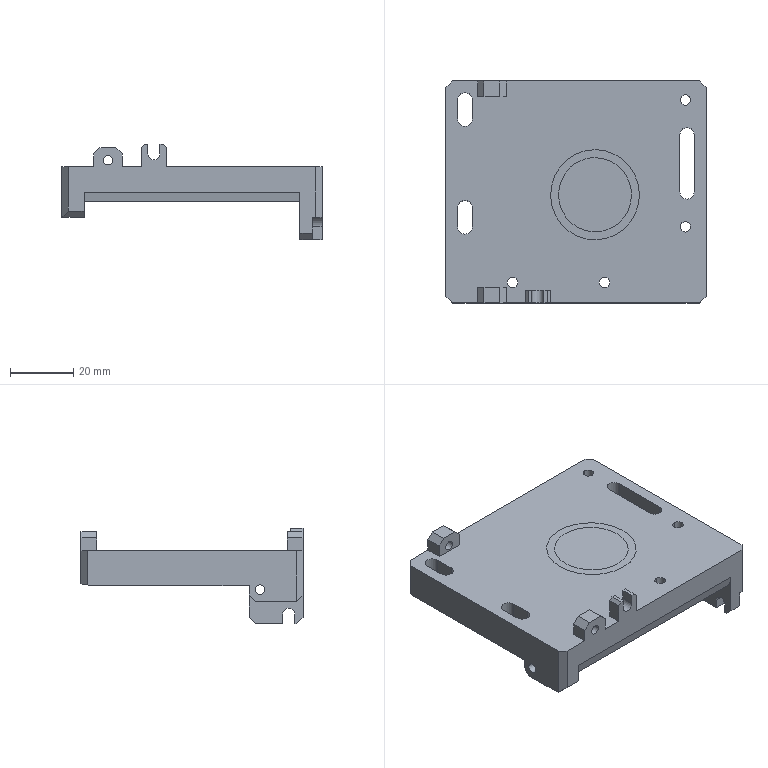NC program | NX | posted with a generic post | part box 82 x 70 x 30 mm
Lines 1 to 2138 of 2435, first 1715 of 2122 lines:
N10 G17 G21 G94 G90
(FLOOR_WALL , TOOL : D10JING)
N12 T11 M6
N14 G54
N16 G17 G0 G90 X45. Y-42.997 B0. C0. S9500 M3
N18 G43 Z30. H11
N20 Z3.
N22 G94 G1 Z0. F1250.
N24 X42.
N26 X-42.
N28 Y-38.174
N30 X42.
N32 Y-33.35
N34 X-42.
N36 Y-28.527
N38 X42.
N40 Y-23.704
N42 X-42.
N44 Y-18.88
N46 X42.
N48 Y-14.057
N50 X-42.
N52 Y-9.234
N54 X42.
N56 Y-4.41
N58 X-42.
N60 Y0.413
N62 X42.
N64 Y5.237
N66 X-42.
N68 Y10.06
N70 X42.
N72 Y14.883
N74 X-42.
N76 Y19.707
N78 X42.
N80 Y24.53
N82 X-42.
N84 Y29.353
N86 X42.
N88 Y34.177
N90 X-42.
N92 Y39.
N94 X42.
N96 X45.
N98 Z3.
N100 G0 Z30.
N102 M5
(FLOOR_WALL_1 , TOOL : D10JING)
N104 M6
N106 G54
N108 G17 G0 G90 X39.14 Y28.025 B0. C0. S9500 M3
N110 G43 Z30. H11
N112 Z-5.5
N114 G94 G1 Z-7. F1250.
N116 X38.866 Y28.5
N118 G3 X38. Y29. R1.
N120 G1 X15.
N122 Y33.
N124 X38.
N126 Y37.
N128 X15.
N130 G3 X14.134 Y36.5 R1.
N132 G1 X13.5 Y35.402
N134 Z-5.5
N136 G0 Z30.
N138 X-38.14 Y46.975
N140 Z-10.5
N142 G1 Z-12.
N144 X-37.866 Y46.5
N146 G3 X-37. Y46. R1.
N148 G1 X12.5
N150 Y41.118
N152 X-37.
N154 Y36.235
N156 X12.5
N158 Y31.353
N160 X-37.
N162 Y26.471
N164 X39.471
N166 Y21.588
N168 X-37.
N170 Y16.706
N172 X39.471
N174 Y11.824
N176 X-37.
N178 Y6.941
N180 X39.471
N182 Y2.059
N184 X-37.
N186 Y-2.824
N188 X39.471
N190 Y-7.706
N192 X-37.
N194 Y-12.588
N196 X39.471
N198 Y-17.471
N200 X-37.
N202 Y-22.353
N204 X39.471
N206 Y-27.235
N208 X-37.
N210 Y-32.118
N212 X12.5
N214 Y-37.
N216 X-37.
N218 Y-41.882
N220 X12.5
N222 G3 X12. Y-41.016 R1.
N224 G1 Z-10.5
N226 G0 Z-1.9
N228 X11.402 Y-47.5
N230 Z-10.5
N232 G1 Z-12.
N234 X12.5 Y-46.866
N236 G3 X13. Y-46. R1.
N238 G1 Y-29.
N240 X39.471
N242 G3 X40.337 Y-28.5 R1.
N244 G1 X40.971 Y-27.402
N246 Z-10.5
N248 G0 Z-1.9
N250 Y27.402
N252 Z-10.5
N254 G1 Z-12.
N256 X40.337 Y28.5
N258 G3 X39.471 Y29. R1.
N260 G1 X13.
N262 Y46.
N264 G3 X12.5 Y46.866 R1.
N266 G1 X11.402 Y47.5
N268 Z-10.5
N270 G0 Z30.
N272 X32.14 Y-46.975
N274 Z1.5
N276 G1 Z0.
N278 X31.866 Y-46.5
N280 G3 X31. Y-46. R1.
N282 G1 X15.
N284 Y-42.
N286 X38.
N288 Y-38.
N290 X15.
N292 G3 X14.134 Y-38.5 R1.
N294 G1 X13.5 Y-39.598
N296 Z1.5
N298 G0 Z30.
N300 X34.671 Y-43.5
N302 Z-5.4
N304 G1 X37.571 Z-6.177
N306 X34.5 Z-7.
N308 X37.571
N310 G2 X38.437 Y-44. R1.
N312 G1 X38.726 Y-44.5
N314 Z-5.5
N316 G0 Z3.1
N318 X39.514
N320 Z-5.5
N322 G1 Z-7.
N324 X38.937 Y-43.5
N326 G3 X38.071 Y-43. R1.
N328 G1 X34.
N330 Y-46.
N332 G3 X34.5 Y-46.866 R1.
N334 G1 X35.5 Y-47.443
N336 Z-5.5
N338 G0 Z30.
(ZLEVEL_PROFILE_COPY , TOOL : D10JING)
N340 X41.809 Y40.622
N342 Z-13.5
N344 G1 Z-15. F1000.
N346 X40.5 Y39.866
N348 G3 X40. Y39. R1.
N350 G1 Y-39. F1200.
N352 G2 X38.536 Y-42.536 R5.
N354 G1 X36.536 Y-44.536
N356 G2 X33. Y-46. R5.
N358 G1 X-33.
N360 G2 X-36.536 Y-44.536 R5.
N362 G1 X-38.536 Y-42.536
N364 G2 X-40. Y-39. R5.
N366 G1 Y39.
N368 G2 X-38.536 Y42.536 R5.
N370 G1 X-36.536 Y44.536
N372 G2 X-33. Y46. R5.
N374 G1 X33.
N376 G2 X36.536 Y44.536 R5.
N378 G1 X38.536 Y42.536
N380 G2 X40. Y39. R5.
N382 G3 X40.5 Y38.134 R1.
N384 G1 X42. Y37.268
N386 Z-13.5
N388 G0 Z30.
N390 X41.809 Y40.622
N392 Z-28.5
N394 G1 Z-30. F1000.
N396 X40.5 Y39.866
N398 G3 X40. Y39. R1.
N400 G1 Y-39. F1200.
N402 G2 X38.536 Y-42.536 R5.
N404 G1 X36.536 Y-44.536
N406 G2 X33. Y-46. R5.
N408 G1 X-33.
N410 G2 X-36.536 Y-44.536 R5.
N412 G1 X-38.536 Y-42.536
N414 G2 X-40. Y-39. R5.
N416 G1 Y39.
N418 G2 X-38.536 Y42.536 R5.
N420 G1 X-36.536 Y44.536
N422 G2 X-33. Y46. R5.
N424 G1 X33.
N426 G2 X36.536 Y44.536 R5.
N428 G1 X38.536 Y42.536
N430 G2 X40. Y39. R5.
N432 G3 X40.5 Y38.134 R1.
N434 G1 X42. Y37.268
N436 Z-28.5
N438 G0 Z30.
N440 M5
(ZLEVEL_PROFILE_COPY_1_COPY , TOOL : D3)
N442 T03 M6
N444 G54
N446 G17 G0 G90 X21. Y-1.698 B0. C0. S9500 M3
N448 G43 Z30. H3
N450 Z-10.5
N452 G94 G1 Y-32.5 Z-12.114 F1000.
N454 X22. Z-12.167
N456 Y32.5 F1200.
N458 X21.
N460 Y-32.5
N462 X22.
N464 Y-22.952 Z-12.333
N466 Y32.5
N468 X21.
N470 Y-32.5
N472 X22.
N474 Y-22.952 Z-12.5
N476 Y32.5
N478 X21.
N480 Y-32.5
N482 X22.
N484 Y-22.952
N486 G3 X21.85 Y-22.692 R0.3
N488 G1 X21.8 Y-22.663
N490 Z-12.2
N492 G0 Z30.
(CAVITY_MILL_COPY , TOOL : D3)
N494 X28.813 Y-41.189
N496 Z1.3
N498 G1 Z-0.2 F1000.
N500 X28.847 Y-40.788
N502 G2 X29.419 Y-39.968 R1.
N504 X31.56 Y-39.807 R3.02 F1100.
N506 G3 X32.178 Y-39.483 R0.5
N508 G2 X30.9 Y-38. R1.5
N510 G1 Y-34.
N512 G2 X32.114 Y-32.528 R1.5
N514 G3 X31.483 Y-32.231 R0.5
N516 G2 X29.517 Y-32.231 R3.02
N518 G3 X28.886 Y-32.528 R0.5
N520 G2 X30.1 Y-34. R1.5
N522 G1 Y-38.
N524 G2 X28.6 Y-39.5 R1.5
N526 G1 X27.499
N528 X27.5 Y-39.536
N530 Y-41.
N532 G2 X27.282 Y-41.778 R1.5
N534 G3 X27.926 Y-41.511 R0.5
N536 G2 X29.419 Y-39.968 R3.02
N538 X30.416 Y-40.053 R1.
N540 G1 X30.745 Y-40.283
N542 Z1.3
N544 G0 X28.813 Y-41.189 Z1.1
N546 G1 Z-0.4 F1000.
N548 X28.847 Y-40.788
N550 G2 X29.419 Y-39.968 R1.
N552 X31.56 Y-39.807 R3.02 F1100.
N554 G3 X32.178 Y-39.483 R0.5
N556 G2 X30.9 Y-38. R1.5
N558 G1 Y-34.
N560 G2 X32.114 Y-32.528 R1.5
N562 G3 X31.483 Y-32.231 R0.5
N564 G2 X29.517 Y-32.231 R3.02
N566 G3 X28.886 Y-32.528 R0.5
N568 G2 X30.1 Y-34. R1.5
N570 G1 Y-38.
N572 G2 X28.6 Y-39.5 R1.5
N574 G1 X27.5
N576 Y-39.536
N578 Y-41.
N580 G2 X27.282 Y-41.778 R1.5
N582 G3 X27.926 Y-41.511 R0.5
N584 G2 X29.419 Y-39.968 R3.02
N586 X30.416 Y-40.053 R1.
N588 G1 X30.745 Y-40.283
N590 Z1.1
N592 G0 X28.813 Y-41.189 Z0.9
N594 G1 Z-0.6 F1000.
N596 X28.847 Y-40.788
N598 G2 X29.419 Y-39.968 R1.
N600 X31.56 Y-39.807 R3.02 F1100.
N602 G3 X32.178 Y-39.483 R0.5
N604 G2 X30.9 Y-38. R1.5
N606 G1 Y-34.
N608 G2 X32.114 Y-32.528 R1.5
N610 G3 X31.483 Y-32.231 R0.5
N612 G2 X29.517 Y-32.231 R3.02
N614 G3 X28.886 Y-32.528 R0.5
N616 G2 X30.1 Y-34. R1.5
N618 G1 Y-38.
N620 G2 X28.6 Y-39.5 R1.5
N622 G1 X27.5
N624 Y-41.
N626 G2 X27.282 Y-41.778 R1.5
N628 G3 X27.926 Y-41.511 R0.5
N630 G2 X29.419 Y-39.968 R3.02
N632 X30.416 Y-40.053 R1.
N634 G1 X30.745 Y-40.283
N636 Z0.9
N638 G0 X28.813 Y-41.189 Z0.7
N640 G1 Z-0.8 F1000.
N642 X28.847 Y-40.788
N644 G2 X29.419 Y-39.968 R1.
N646 X31.56 Y-39.807 R3.02 F1100.
N648 G3 X32.178 Y-39.483 R0.5
N650 G2 X30.9 Y-38. R1.5
N652 G1 Y-34.
N654 G2 X32.114 Y-32.528 R1.5
N656 G3 X31.483 Y-32.231 R0.5
N658 G2 X29.517 Y-32.231 R3.02
N660 G3 X28.886 Y-32.528 R0.5
N662 G2 X30.1 Y-34. R1.5
N664 G1 Y-38.
N666 G2 X28.6 Y-39.5 R1.5
N668 G1 X27.5
N670 Y-41.
N672 G2 X27.282 Y-41.778 R1.5
N674 G3 X27.926 Y-41.511 R0.5
N676 G2 X29.419 Y-39.968 R3.02
N678 X30.416 Y-40.053 R1.
N680 G1 X30.745 Y-40.283
N682 Z0.7
N684 G0 X28.813 Y-41.189 Z0.5
N686 G1 Z-1. F1000.
N688 X28.847 Y-40.788
N690 G2 X29.419 Y-39.968 R1.
N692 X31.56 Y-39.807 R3.02 F1100.
N694 G3 X32.178 Y-39.483 R0.5
N696 G2 X30.9 Y-38. R1.5
N698 G1 Y-34.
N700 G2 X32.114 Y-32.528 R1.5
N702 G3 X31.483 Y-32.231 R0.5
N704 G2 X29.517 Y-32.231 R3.02
N706 G3 X28.886 Y-32.528 R0.5
N708 G2 X30.1 Y-34. R1.5
N710 G1 Y-38.
N712 G2 X28.6 Y-39.5 R1.5
N714 G1 X27.5
N716 Y-41.
N718 G2 X27.282 Y-41.778 R1.5
N720 G3 X27.926 Y-41.511 R0.5
N722 G2 X29.419 Y-39.968 R3.02
N724 X30.416 Y-40.053 R1.
N726 G1 X30.745 Y-40.283
N728 Z0.5
N730 G0 X28.813 Y-41.189 Z0.3
N732 G1 Z-1.2 F1000.
N734 X28.847 Y-40.788
N736 G2 X29.419 Y-39.968 R1.
N738 X31.56 Y-39.807 R3.02 F1100.
N740 G3 X32.178 Y-39.483 R0.5
N742 G2 X30.9 Y-38. R1.5
N744 G1 Y-34.
N746 G2 X32.114 Y-32.528 R1.5
N748 G3 X31.483 Y-32.231 R0.5
N750 G2 X29.517 Y-32.231 R3.02
N752 G3 X28.886 Y-32.528 R0.5
N754 G2 X30.1 Y-34. R1.5
N756 G1 Y-38.
N758 G2 X28.6 Y-39.5 R1.5
N760 G1 X27.5
N762 Y-41.
N764 G2 X27.282 Y-41.778 R1.5
N766 G3 X27.926 Y-41.511 R0.5
N768 G2 X29.419 Y-39.968 R3.02
N770 X30.416 Y-40.053 R1.
N772 G1 X30.745 Y-40.283
N774 Z0.3
N776 G0 X28.813 Y-41.189 Z0.1
N778 G1 Z-1.4 F1000.
N780 X28.847 Y-40.788
N782 G2 X29.419 Y-39.968 R1.
N784 X31.56 Y-39.807 R3.02 F1100.
N786 G3 X32.178 Y-39.483 R0.5
N788 G2 X30.9 Y-38. R1.5
N790 G1 Y-34.
N792 G2 X32.114 Y-32.528 R1.5
N794 G3 X31.483 Y-32.231 R0.5
N796 G2 X29.517 Y-32.231 R3.02
N798 G3 X28.886 Y-32.528 R0.5
N800 G2 X30.1 Y-34. R1.5
N802 G1 Y-38.
N804 G2 X28.6 Y-39.5 R1.5
N806 G1 X27.5
N808 Y-41.
N810 G2 X27.282 Y-41.778 R1.5
N812 G3 X27.926 Y-41.511 R0.5
N814 G2 X29.419 Y-39.968 R3.02
N816 X30.416 Y-40.053 R1.
N818 G1 X30.745 Y-40.283
N820 Z0.1
N822 G0 X28.813 Y-41.189 Z-0.1
N824 G1 Z-1.6 F1000.
N826 X28.847 Y-40.788
N828 G2 X29.419 Y-39.968 R1.
N830 X31.56 Y-39.807 R3.02 F1100.
N832 G3 X32.178 Y-39.483 R0.5
N834 G2 X30.9 Y-38. R1.5
N836 G1 Y-34.
N838 G2 X32.114 Y-32.528 R1.5
N840 G3 X31.483 Y-32.231 R0.5
N842 G2 X29.517 Y-32.231 R3.02
N844 G3 X28.886 Y-32.528 R0.5
N846 G2 X30.1 Y-34. R1.5
N848 G1 Y-38.
N850 G2 X28.6 Y-39.5 R1.5
N852 G1 X27.503
N854 X27.5 Y-39.536
N856 Y-41.
N858 G2 X27.282 Y-41.778 R1.5
N860 G3 X27.926 Y-41.511 R0.5
N862 G2 X29.419 Y-39.968 R3.02
N864 X30.416 Y-40.053 R1.
N866 G1 X30.745 Y-40.283
N868 Z-0.1
N870 G0 X28.813 Y-41.189 Z-0.3
N872 G1 Z-1.8 F1000.
N874 X28.847 Y-40.788
N876 G2 X29.419 Y-39.968 R1.
N878 X31.56 Y-39.807 R3.02 F1100.
N880 G3 X32.178 Y-39.483 R0.5
N882 G2 X30.9 Y-38. R1.5
N884 G1 Y-34.
N886 G2 X32.114 Y-32.528 R1.5
N888 G3 X31.483 Y-32.231 R0.5
N890 G2 X29.517 Y-32.231 R3.02
N892 G3 X28.886 Y-32.528 R0.5
N894 G2 X30.1 Y-34. R1.5
N896 G1 Y-38.
N898 G2 X28.6 Y-39.5 R1.5
N900 G1 X27.504
N902 X27.5 Y-39.536
N904 Y-41.
N906 G2 X27.282 Y-41.778 R1.5
N908 G3 X27.926 Y-41.511 R0.5
N910 G2 X29.419 Y-39.968 R3.02
N912 X30.416 Y-40.053 R1.
N914 G1 X30.745 Y-40.283
N916 Z-0.3
N918 G0 X28.813 Y-41.189 Z-0.5
N920 G1 Z-2. F1000.
N922 X28.847 Y-40.788
N924 G2 X29.419 Y-39.968 R1.
N926 X31.56 Y-39.807 R3.02 F1100.
N928 G3 X32.178 Y-39.483 R0.5
N930 G2 X30.9 Y-38. R1.5
N932 G1 Y-34.
N934 G2 X32.114 Y-32.528 R1.5
N936 G3 X31.483 Y-32.231 R0.5
N938 G2 X29.517 Y-32.231 R3.02
N940 G3 X28.886 Y-32.528 R0.5
N942 G2 X30.1 Y-34. R1.5
N944 G1 Y-38.
N946 G2 X28.6 Y-39.5 R1.5
N948 G1 X27.505
N950 X27.5 Y-39.536
N952 Y-41.
N954 G2 X27.282 Y-41.778 R1.5
N956 G3 X27.926 Y-41.511 R0.5
N958 G2 X29.419 Y-39.968 R3.02
N960 X30.416 Y-40.053 R1.
N962 G1 X30.745 Y-40.283
N964 Z-0.5
N966 G0 X28.813 Y-41.189 Z-0.7
N968 G1 Z-2.2 F1000.
N970 X28.847 Y-40.788
N972 G2 X29.419 Y-39.968 R1.
N974 X31.56 Y-39.807 R3.02 F1100.
N976 G3 X32.178 Y-39.483 R0.5
N978 G2 X30.9 Y-38. R1.5
N980 G1 Y-34.
N982 G2 X32.114 Y-32.528 R1.5
N984 G3 X31.483 Y-32.231 R0.5
N986 G2 X29.517 Y-32.231 R3.02
N988 G3 X28.886 Y-32.528 R0.5
N990 G2 X30.1 Y-34. R1.5
N992 G1 Y-38.
N994 G2 X28.6 Y-39.5 R1.5
N996 G1 X27.506
N998 X27.5 Y-39.536
N1000 Y-41.
N1002 G2 X27.282 Y-41.778 R1.5
N1004 G3 X27.926 Y-41.511 R0.5
N1006 G2 X29.419 Y-39.968 R3.02
N1008 X30.416 Y-40.053 R1.
N1010 G1 X30.745 Y-40.283
N1012 Z-0.7
N1014 G0 X28.813 Y-41.189 Z-0.9
N1016 G1 Z-2.4 F1000.
N1018 X28.847 Y-40.788
N1020 G2 X29.419 Y-39.968 R1.
N1022 X31.56 Y-39.807 R3.02 F1100.
N1024 G3 X32.178 Y-39.483 R0.5
N1026 G2 X30.9 Y-38. R1.5
N1028 G1 Y-34.
N1030 G2 X32.114 Y-32.528 R1.5
N1032 G3 X31.483 Y-32.231 R0.5
N1034 G2 X29.517 Y-32.231 R3.02
N1036 G3 X28.886 Y-32.528 R0.5
N1038 G2 X30.1 Y-34. R1.5
N1040 G1 Y-38.
N1042 G2 X28.6 Y-39.5 R1.5
N1044 G1 X27.5
N1046 Y-41.
N1048 G2 X27.282 Y-41.778 R1.5
N1050 G3 X27.926 Y-41.511 R0.5
N1052 G2 X29.419 Y-39.968 R3.02
N1054 X30.416 Y-40.053 R1.
N1056 G1 X30.745 Y-40.283
N1058 Z-0.9
N1060 G0 X28.813 Y-41.189 Z-1.1
N1062 G1 Z-2.6 F1000.
N1064 X28.847 Y-40.788
N1066 G2 X29.419 Y-39.968 R1.
N1068 X31.56 Y-39.807 R3.02 F1100.
N1070 G3 X32.178 Y-39.483 R0.5
N1072 G2 X30.9 Y-38. R1.5
N1074 G1 Y-34.
N1076 G2 X32.114 Y-32.528 R1.5
N1078 G3 X31.483 Y-32.231 R0.5
N1080 G2 X29.517 Y-32.231 R3.02
N1082 G3 X28.886 Y-32.528 R0.5
N1084 G2 X30.1 Y-34. R1.5
N1086 G1 Y-38.
N1088 G2 X28.6 Y-39.5 R1.5
N1090 G1 X27.5
N1092 Y-41.
N1094 G2 X27.282 Y-41.778 R1.5
N1096 G3 X27.926 Y-41.511 R0.5
N1098 G2 X29.419 Y-39.968 R3.02
N1100 X30.416 Y-40.053 R1.
N1102 G1 X30.745 Y-40.283
N1104 Z-1.1
N1106 G0 X28.813 Y-41.189 Z-1.3
N1108 G1 Z-2.8 F1000.
N1110 X28.847 Y-40.788
N1112 G2 X29.419 Y-39.968 R1.
N1114 X31.56 Y-39.807 R3.02 F1100.
N1116 G3 X32.178 Y-39.483 R0.5
N1118 G2 X30.9 Y-38. R1.5
N1120 G1 Y-34.
N1122 G2 X32.114 Y-32.528 R1.5
N1124 G3 X31.483 Y-32.231 R0.5
N1126 G2 X29.517 Y-32.231 R3.02
N1128 G3 X28.886 Y-32.528 R0.5
N1130 G2 X30.1 Y-34. R1.5
N1132 G1 Y-38.
N1134 G2 X28.6 Y-39.5 R1.5
N1136 G1 X27.5
N1138 Y-41.
N1140 G2 X27.282 Y-41.778 R1.5
N1142 G3 X27.926 Y-41.511 R0.5
N1144 G2 X29.419 Y-39.968 R3.02
N1146 X30.416 Y-40.053 R1.
N1148 G1 X30.745 Y-40.283
N1150 Z-1.3
N1152 G0 X28.813 Y-41.189 Z-1.5
N1154 G1 Z-3. F1000.
N1156 X28.847 Y-40.788
N1158 G2 X29.419 Y-39.968 R1.
N1160 X31.56 Y-39.807 R3.02 F1100.
N1162 G3 X32.178 Y-39.483 R0.5
N1164 G2 X30.9 Y-38. R1.5
N1166 G1 Y-34.
N1168 G2 X32.114 Y-32.528 R1.5
N1170 G3 X31.483 Y-32.231 R0.5
N1172 G2 X29.517 Y-32.231 R3.02
N1174 G3 X28.886 Y-32.528 R0.5
N1176 G2 X30.1 Y-34. R1.5
N1178 G1 Y-38.
N1180 G2 X28.6 Y-39.5 R1.5
N1182 G1 X27.5
N1184 Y-41.
N1186 G2 X27.282 Y-41.778 R1.5
N1188 G3 X27.926 Y-41.511 R0.5
N1190 G2 X29.419 Y-39.968 R3.02
N1192 X30.416 Y-40.053 R1.
N1194 G1 X30.745 Y-40.283
N1196 Z-1.5
N1198 G0 X28.813 Y-41.193 Z-1.7
N1200 G1 Z-3.2 F1000.
N1202 X28.848 Y-40.793
N1204 G2 X29.422 Y-39.974 R1.
N1206 X31.458 Y-39.788 R3.02 F1100.
N1208 G1 X31.556 Y-39.815
N1210 G3 X32.171 Y-39.486 R0.5
N1212 G2 X30.889 Y-38. R1.487
N1214 G1 Y-34.
N1216 G2 X32.088 Y-32.528 R1.486
N1218 G3 X31.462 Y-32.232 R0.5
N1220 G2 X29.945 Y-32.337 R3.02
N1222 X29.534 Y-32.231 R3.02
N1224 G3 X28.907 Y-32.53 R0.5
N1226 G2 X30.099 Y-33.827 R1.475
N1228 G1 X30.117 Y-33.999
N1230 X30.111 Y-34.02
N1232 Y-38.
N1234 G2 X28.6 Y-39.5 R1.483
N1236 G1 X27.5
N1238 Y-41.
N1240 G2 X27.281 Y-41.781 R1.5
N1242 G3 X27.925 Y-41.514 R0.5
N1244 G2 X29.422 Y-39.974 R3.02
N1246 X30.418 Y-40.061 R1.
N1248 G1 X30.747 Y-40.292
N1250 Z-1.7
N1252 G0 X28.813 Y-41.196 Z-1.9
N1254 G1 Z-3.4 F1000.
N1256 X28.849 Y-40.796
N1258 G2 X29.424 Y-39.978 R1.
N1260 X31.52 Y-39.812 R3.02 F1100.
N1262 G3 X32.132 Y-39.485 R0.5
N1264 G2 X30.894 Y-38.349 R1.496
N1266 G1 X30.85 Y-38.105
N1268 X30.857 Y-38.
N1270 Y-34.011
N1272 X30.846 Y-33.988
N1274 G2 X31.374 Y-32.863 R1.55
N1276 G1 X31.553 Y-32.731
N1278 G2 X32.093 Y-32.516 R1.324
N1280 G3 X31.464 Y-32.212 R0.5
N1282 G2 X29.533 Y-32.21 R3.02
N1284 G3 X28.9 Y-32.519 R0.5
N1286 G2 X30.143 Y-34.033 R1.49
N1288 G1 Y-38.
N1290 G2 X28.713 Y-39.499 R1.482
N1292 G1 X28.6 Y-39.5
N1294 X27.5
N1296 Y-41.
N1298 G2 X27.28 Y-41.782 R1.5
N1300 G3 X27.925 Y-41.517 R0.5
N1302 G2 X29.424 Y-39.978 R3.02
N1304 X30.42 Y-40.067 R1.
N1306 G1 X30.749 Y-40.298
N1308 Z-1.9
N1310 G0 X28.814 Y-41.206 Z-2.1
N1312 G1 Z-3.6 F1000.
N1314 X28.851 Y-40.806
N1316 G2 X29.43 Y-39.99 R1.
N1318 X31.483 Y-39.821 R3.02 F1100.
N1320 G3 X32.091 Y-39.487 R0.5
N1322 G2 X30.835 Y-38.349 R1.495
N1324 G1 X30.798 Y-38.105
N1326 X30.803 Y-38.
N1328 Y-34.029
N1330 X30.794 Y-33.993
N1332 G2 X30.886 Y-33.489 R1.196
N1334 X32.044 Y-32.52 R1.489
N1336 G3 X31.42 Y-32.207 R0.5
N1338 G2 X29.582 Y-32.207 R3.02
N1340 G3 X28.957 Y-32.52 R0.5
N1342 G2 X30.153 Y-33.621 R1.483
N1344 G1 X30.184 Y-33.708
N1346 G2 X30.206 Y-34. R2.036
N1348 G1 X30.197 Y-34.03
N1350 Y-38.
N1352 X30.202 Y-38.105
N1354 G2 X30.153 Y-38.39 R0.68
N1356 X28.706 Y-39.5 R1.489
N1358 G1 X27.5
N1360 Y-41.
N1362 G2 X27.277 Y-41.787 R1.5
N1364 G3 X27.923 Y-41.524 R0.5
N1366 G2 X29.43 Y-39.99 R3.02
N1368 X30.425 Y-40.083 R1.
N1370 G1 X30.753 Y-40.316
N1372 Z-2.1
N1374 G0 X28.814 Y-41.218 Z-2.3
N1376 G1 Z-3.8 F1000.
N1378 X28.854 Y-40.819
N1380 G2 X29.437 Y-40.006 R1.
N1382 X31.437 Y-39.835 R3.02 F1100.
N1384 G3 X32.042 Y-39.49 R0.5
N1386 G2 X30.717 Y-37.965 R1.498
N1388 G1 X30.723 Y-37.948
N1390 Y-34.049
N1392 X30.717 Y-34.037
N1394 X30.714 Y-33.952
N1396 G2 X31.988 Y-32.517 R1.501
N1398 G3 X31.37 Y-32.195 R0.5
N1400 G2 X29.629 Y-32.194 R3.02
N1402 G3 X29.01 Y-32.517 R0.5
N1404 G2 X30.184 Y-33.464 R1.493
N1406 G1 X30.261 Y-33.708
N1408 G2 X30.284 Y-33.996 R1.975
N1410 G1 X30.277 Y-34.037
N1412 Y-37.949
N1414 X30.283 Y-37.966
N1416 G2 X30.161 Y-38.593 R1.286
N1418 X28.784 Y-39.5 R1.496
N1420 G1 X27.5
N1422 Y-41.
N1424 G2 X27.273 Y-41.793 R1.5
N1426 G3 X27.92 Y-41.534 R0.5
N1428 G2 X29.437 Y-40.006 R3.02
N1430 X30.432 Y-40.106 R1.
N1432 G1 X30.758 Y-40.34
N1434 Z-2.3
N1436 G0 X28.814 Y-41.235 Z-2.5
N1438 G1 Z-4. F1000.
N1440 X28.857 Y-40.836
N1442 G2 X29.447 Y-40.028 R1.
N1444 X31.369 Y-39.853 R3.02 F1100.
N1446 G3 X31.968 Y-39.494 R0.5
N1448 G2 X30.61 Y-37.965 R1.493
N1450 G1 X30.616 Y-37.948
N1452 Y-34.049
N1454 X30.61 Y-34.037
N1456 G2 X30.702 Y-33.464 R1.679
N1458 X31.921 Y-32.512 R1.51
N1460 G3 X31.309 Y-32.174 R0.5
N1462 G2 X29.697 Y-32.175 R3.02
N1464 G3 X29.085 Y-32.512 R0.5
N1466 G2 X30.39 Y-34.021 R1.493
N1468 G1 X30.384 Y-34.032
N1470 Y-37.948
N1472 X30.39 Y-37.965
N1474 G2 X28.89 Y-39.5 R1.496
N1476 G1 X27.507
N1478 X27.5 Y-39.522
N1480 Y-41.
N1482 G2 X27.268 Y-41.802 R1.5
N1484 G3 X27.916 Y-41.547 R0.5
N1486 G2 X29.447 Y-40.028 R3.02
N1488 X30.441 Y-40.135 R1.
N1490 G1 X30.765 Y-40.372
N1492 Z-2.5
N1494 G0 X32.749 Y-40.1 Z-2.7
N1496 G1 Z-4.2 F1000.
N1498 X32.721 Y-40.044
N1500 G3 X31.883 Y-39.498 R1.
N1502 G2 X30.5 Y-38.337 R1.505 F1100.
N1504 X29.039 Y-39.5 R1.504
N1506 G1 X27.507
N1508 Y-40.973
N1510 X27.513 Y-40.985
N1512 X27.486 Y-41.28
N1514 X27.468 Y-41.352
N1516 G2 X27.27 Y-41.82 R1.456
N1518 G3 X27.185 Y-42.742 R1.
N1520 G1 Z-2.7
N1522 G0 X32.639 Y-40.1 Z-2.9
N1524 G1 Z-4.4 F1000.
N1526 X32.596 Y-40.021
N1528 G3 X31.743 Y-39.5 R1.
N1530 G2 X30.502 Y-38.792 R1.509 F1100.
N1532 X29.225 Y-39.5 R1.518
N1534 G1 X27.527
N1536 Y-40.984
N1538 G2 X27.292 Y-41.818 R1.478
N1540 G3 X27.209 Y-42.742 R1.
N1542 G1 Z-2.9
N1544 G0 X32.481 Y-40.1 Z-3.1
N1546 G1 Z-4.6 F1000.
N1548 X32.423 Y-40.
N1550 G3 X31.557 Y-39.5 R1.
N1552 G1 X31.518 F1100.
N1554 G2 X30.502 Y-39.101 R1.476
N1556 X29.482 Y-39.5 R1.511
N1558 G1 X27.561
N1560 Y-40.969
N1562 X27.568 Y-41.036
N1564 G2 X27.314 Y-41.838 R1.498
N1566 G3 X27.213 Y-42.762 R1.
N1568 G1 Z-3.1
N1570 G0 X32.192 Y-40.1 Z-3.3
N1572 G1 Z-4.8 F1000.
N1574 X32.134 Y-40.
N1576 G3 X31.268 Y-39.5 R1.
N1578 G1 X31.08 F1100.
N1580 G2 X30.502 Y-39.375 R1.423
N1582 X29.92 Y-39.5 R1.536
N1584 G1 X27.609
N1586 Y-40.978
N1588 X27.617 Y-41.036
N1590 X27.602 Y-41.175
N1592 G2 X27.34 Y-41.867 R1.489
N1594 G3 X27.22 Y-42.788 R1.
N1596 G1 Z-3.3
N1598 G0 X31.809 Y-40.1 Z-3.5
N1600 G1 Z-5. F1000.
N1602 X31.751 Y-40.
N1604 G3 X30.885 Y-39.5 R1.
N1606 G1 X27.672 F1100.
N1608 Y-40.961
N1610 X27.677 Y-40.988
N1612 G2 X27.413 Y-41.854 R1.494
N1614 G3 X27.302 Y-42.776 R1.
N1616 G1 Z-3.5
N1618 G0 X31.891 Y-40.1 Z-3.7
N1620 G1 Z-5.2 F1000.
N1622 X31.834 Y-40.
N1624 G3 X30.968 Y-39.5 R1.
N1626 G1 X27.75 F1100.
N1628 Y-41.
N1630 X27.76 Y-41.036
N1632 G2 X27.492 Y-41.856 R1.502
N1634 G3 X27.376 Y-42.779 R1.
N1636 G1 Z-3.7
N1638 G0 X31.981 Y-40.1 Z-3.9
N1640 G1 Z-5.4 F1000.
N1642 X31.923 Y-40.
N1644 G3 X31.057 Y-39.5 R1.
N1646 G1 X27.847 F1100.
N1648 Y-41.
N1650 G2 X27.589 Y-41.854 R1.482
N1652 G3 X27.481 Y-42.776 R1.
N1654 G1 Z-3.9
N1656 G0 X32.104 Y-40.1 Z-4.1
N1658 G1 Z-5.6 F1000.
N1660 X32.047 Y-40.
N1662 G3 X31.181 Y-39.5 R1.
N1664 G1 X27.962 F1100.
N1666 Y-41.
N1668 X27.973 Y-41.036
N1670 G2 X27.7 Y-41.86 R1.503
N1672 G3 X27.581 Y-42.783 R1.
N1674 G1 Z-4.1
N1676 G0 X32.247 Y-40.1 Z-4.3
N1678 G1 Z-5.8 F1000.
N1680 X32.189 Y-40.
N1682 G3 X31.323 Y-39.5 R1.
N1684 G1 X28.1 F1100.
N1686 Y-41.
N1688 G2 X27.797 Y-41.912 R1.487
N1690 G3 X27.643 Y-42.828 R1.
N1692 G1 Z-4.3
N1694 G0 X32.407 Y-40.1 Z-4.5
N1696 G1 Z-6. F1000.
N1698 X32.349 Y-40.
N1700 G3 X31.483 Y-39.5 R1.
N1702 G1 X28.264 F1100.
N1704 Y-40.974
N1706 X28.281 Y-41.036
N1708 G2 X28.2 Y-41.454 R1.102
N1710 X27.999 Y-41.863 R1.493
N1712 G3 X27.881 Y-42.785 R1.
N1714 G1 Z-4.5
N1716 G0 X32.604 Y-40.1 Z-4.7
N1718 G1 Z-6.2 F1000.
N1720 X32.546 Y-40.
N1722 G3 X31.68 Y-39.5 R1.
N1724 G1 X28.46 F1100.
N1726 Y-40.974
N1728 X28.47 Y-41.036
N1730 G2 X28.202 Y-41.859 R1.488
N1732 G3 X28.085 Y-42.78 R1.
N1734 G1 Z-4.7
N1736 G0 X32.837 Y-40.1 Z-4.9
N1738 G1 Z-6.4 F1000.
N1740 X32.78 Y-40.
N1742 G3 X31.914 Y-39.5 R1.
N1744 G1 X28.7 F1100.
N1746 Y-41.
N1748 G2 X28.438 Y-41.862 R1.478
N1750 G3 X28.326 Y-42.783 R1.
N1752 G1 Z-4.9
N1754 G0 X33.151 Y-40.1 Z-5.1
N1756 G1 Z-6.6 F1000.
N1758 X33.093 Y-40.
N1760 G3 X32.227 Y-39.5 R1.
N1762 G1 X29.003 F1100.
N1764 Y-40.974
N1766 X29.023 Y-41.036
N1768 G2 X28.808 Y-41.769 R1.535
N1770 G1 X28.754 Y-41.854
N1772 G3 X28.641 Y-42.776 R1.
N1774 G1 Z-5.1
N1776 G0 X33.583 Y-40.1 Z-5.3
N1778 G1 Z-6.8 F1000.
N1780 X33.525 Y-40.
N1782 G3 X32.659 Y-39.5 R1.
N1784 G1 X29.423 F1100.
N1786 Y-40.974
N1788 X29.449 Y-41.036
N1790 G2 X29.35 Y-41.524 R1.776
N1792 X29.146 Y-41.89 R1.534
N1794 G3 X28.996 Y-42.81 R1.
N1796 G1 Z-5.3
N1798 G0 X34.566 Y-40.1 Z-5.5
N1800 G1 Z-7. F1000.
N1802 X34.509 Y-40.
N1804 G3 X33.643 Y-39.5 R1.
N1806 G1 X30.378 F1100.
N1808 Y-41.
N1810 X30.406 Y-40.987
N1812 X30.435 Y-41.004
N1814 X30.436 Y-41.036
N1816 G2 X30.19 Y-41.814 R1.237
N1818 G3 X30.049 Y-42.753 R1.
N1820 G1 Z-5.5
N1822 G0 Z30.
N1824 X28.339 Y-31.9
N1826 Z-2.7
N1828 G1 Z-4.2 F1000.
N1830 X28.353 Y-31.931
N1832 G3 X29.172 Y-32.506 R1.
N1834 G2 X30.498 Y-33.666 R1.495 F1100.
N1836 X31.831 Y-32.506 R1.504
N1838 G3 X32.649 Y-31.931 R1.
N1840 G1 X32.664 Y-31.9
N1842 Z-2.7
N1844 G0 X28.456 Z-2.9
N1846 G1 Z-4.4 F1000.
N1848 X28.482 Y-31.952
N1850 G3 X29.317 Y-32.503 R1.
N1852 G2 X30.498 Y-33.209 R1.492 F1100.
N1854 X31.687 Y-32.503 R1.51
N1856 G3 X32.522 Y-31.952 R1.
N1858 G1 X32.548 Y-31.9
N1860 Z-2.9
N1862 G0 X28.572 Z-3.1
N1864 G1 Z-4.6 F1000.
N1866 X28.628 Y-31.997
N1868 G3 X29.492 Y-32.5 R1.
N1870 G2 X30.498 Y-32.897 R1.486 F1100.
N1872 X31.525 Y-32.5 R1.503
N1874 G3 X32.394 Y-32.005 R1.
N1876 G1 X32.456 Y-31.9
N1878 Z-3.1
N1880 G0 X28.82 Z-3.3
N1882 G1 Z-4.8 F1000.
N1884 X28.878 Y-32.
N1886 G3 X29.744 Y-32.5 R1.
N1888 G1 X29.92 F1100.
N1890 G2 X30.519 Y-32.609 R3.215
N1892 X31.08 Y-32.5 R1.862
N1894 G1 X31.235
N1896 G3 X32.101 Y-32. R1.
N1898 G1 X32.158 Y-31.9
N1900 Z-3.3
N1902 G0 Z30.
N1904 M5
(CAVITY_MILL_COPY_COPY_COPY , TOOL : D1.5)
N1906 T14 M6
N1908 G54
N1910 G17 G0 G90 X20.55 Y-31.46 B0. C0. S9500 M3
N1912 G43 Z30. H14
N1914 Z-10.6
N1916 G94 G1 Z-12.1 F1000.
N1918 G3 X20.25 Y-32.174 R1.
N1920 G1 Y-33. F1100.
N1922 G3 X20.5 Y-33.25 R0.25
N1924 G1 X21.326
N1926 G3 X21.576 Y-33.183 R0.5
N1928 G1 X21.5 Y-32.82
N1930 Z-10.6
N1932 G0 Z30.
N1934 X20.55 Y-31.46
N1936 Z-10.7
N1938 G1 Z-12.2 F1000.
N1940 G3 X20.25 Y-32.174 R1.
N1942 G1 Y-33. F1100.
N1944 G3 X20.5 Y-33.25 R0.25
N1946 G1 X21.326
N1948 G3 X21.576 Y-33.183 R0.5
N1950 G1 X21.5 Y-32.82
N1952 Z-10.7
N1954 G0 Z30.
N1956 X20.55 Y-31.46
N1958 Z-10.8
N1960 G1 Z-12.3 F1000.
N1962 G3 X20.25 Y-32.174 R1.
N1964 G1 Y-33. F1100.
N1966 G3 X20.5 Y-33.25 R0.25
N1968 G1 X21.326
N1970 G3 X21.576 Y-33.183 R0.5
N1972 G1 X21.5 Y-32.82
N1974 Z-10.8
N1976 G0 Z30.
N1978 X20.55 Y-31.46
N1980 Z-10.9
N1982 G1 Z-12.4 F1000.
N1984 G3 X20.25 Y-32.174 R1.
N1986 G1 Y-33. F1100.
N1988 G3 X20.5 Y-33.25 R0.25
N1990 G1 X21.326
N1992 G3 X21.576 Y-33.183 R0.5
N1994 G1 X21.5 Y-32.82
N1996 Z-10.9
N1998 G0 Z30.
N2000 X20.55 Y-31.46
N2002 Z-11.
N2004 G1 Z-12.5 F1000.
N2006 G3 X20.25 Y-32.174 R1.
N2008 G1 Y-33. F1100.
N2010 G3 X20.5 Y-33.25 R0.25
N2012 G1 X21.326
N2014 G3 X21.576 Y-33.183 R0.5
N2016 G1 X21.5 Y-32.82
N2018 Z-11.
N2020 G0 Z30.
N2022 X21.025 Y-32.475
N2024 Z-10.6
N2026 G1 Z-12.1 F1000.
N2028 X20.808 Y-32.75
N2030 G3 X21.674 Y-33.25 R1.
N2032 G1 X22.5 F1100.
N2034 G3 X22.75 Y-33. R0.25
N2036 G1 Y-32.174
N2038 G3 X22.45 Y-31.46 R1.
N2040 G1 Z-10.6
N2042 G0 Z30.
N2044 X21.025 Y-32.475
N2046 Z-10.7
N2048 G1 Z-12.2 F1000.
N2050 X20.808 Y-32.75
N2052 G3 X21.674 Y-33.25 R1.
N2054 G1 X22.5 F1100.
N2056 G3 X22.75 Y-33. R0.25
N2058 G1 Y-32.174
N2060 G3 X22.45 Y-31.46 R1.
N2062 G1 Z-10.7
N2064 G0 Z30.
N2066 X21.025 Y-32.475
N2068 Z-10.8
N2070 G1 Z-12.3 F1000.
N2072 X20.808 Y-32.75
N2074 G3 X21.674 Y-33.25 R1.
N2076 G1 X22.5 F1100.
N2078 G3 X22.75 Y-33. R0.25
N2080 G1 Y-32.174
N2082 G3 X22.45 Y-31.46 R1.
N2084 G1 Z-10.8
N2086 G0 Z30.
N2088 X21.025 Y-32.475
N2090 Z-10.9
N2092 G1 Z-12.4 F1000.
N2094 X20.808 Y-32.75
N2096 G3 X21.674 Y-33.25 R1.
N2098 G1 X22.5 F1100.
N2100 G3 X22.75 Y-33. R0.25
N2102 G1 Y-32.174
N2104 G3 X22.45 Y-31.46 R1.
N2106 G1 Z-10.9
N2108 G0 Z30.
N2110 X21.025 Y-32.475
N2112 Z-11.
N2114 G1 Z-12.5 F1000.
N2116 X20.808 Y-32.75
N2118 G3 X21.674 Y-33.25 R1.
N2120 G1 X22.5 F1100.
N2122 G3 X22.75 Y-33. R0.25
N2124 G1 Y-32.174
N2126 G3 X22.45 Y-31.46 R1.
N2128 G1 Z-11.
N2130 G0 Z30.
N2132 Y31.46
N2134 Z-10.6
N2136 G1 Z-12.1 F1000.
N2138 G3 X22.75 Y32.174 R1.
N2140 G1 Y33. F1100.
N2142 G3 X22.5 Y33.25 R0.25
N2144 G1 X21.674
N2146 G3 X21.424 Y33.183 R0.5
N2148 G1 X21.5 Y32.82
N2150 Z-10.6
N2152 G0 Z30.
N2154 X22.45 Y31.46
N2156 Z-10.7
N2158 G1 Z-12.2 F1000.
N2160 G3 X22.75 Y32.174 R1.
N2162 G1 Y33. F1100.
N2164 G3 X22.5 Y33.25 R0.25
N2166 G1 X21.674
N2168 G3 X21.424 Y33.183 R0.5
N2170 G1 X21.5 Y32.82
N2172 Z-10.7
N2174 G0 Z30.
N2176 X22.45 Y31.46
N2178 Z-10.8
N2180 G1 Z-12.3 F1000.
N2182 G3 X22.75 Y32.174 R1.
N2184 G1 Y33. F1100.
N2186 G3 X22.5 Y33.25 R0.25
N2188 G1 X21.674
N2190 G3 X21.424 Y33.183 R0.5
N2192 G1 X21.5 Y32.82
N2194 Z-10.8
N2196 G0 Z30.
N2198 X22.45 Y31.46
N2200 Z-10.9
N2202 G1 Z-12.4 F1000.
N2204 G3 X22.75 Y32.174 R1.
N2206 G1 Y33. F1100.
N2208 G3 X22.5 Y33.25 R0.25
N2210 G1 X21.674
N2212 G3 X21.424 Y33.183 R0.5
N2214 G1 X21.5 Y32.82
N2216 Z-10.9
N2218 G0 Z30.
N2220 X22.45 Y31.46
N2222 Z-11.
N2224 G1 Z-12.5 F1000.
N2226 G3 X22.75 Y32.174 R1.
N2228 G1 Y33. F1100.
N2230 G3 X22.5 Y33.25 R0.25
N2232 G1 X21.674
N2234 G3 X21.424 Y33.183 R0.5
N2236 G1 X21.5 Y32.82
N2238 Z-11.
N2240 G0 Z30.
N2242 X21.975 Y32.475
N2244 Z-10.6
N2246 G1 Z-12.1 F1000.
N2248 X22.192 Y32.75
N2250 G3 X21.326 Y33.25 R1.
N2252 G1 X20.5 F1100.
N2254 G3 X20.25 Y33. R0.25
N2256 G1 Y32.174
N2258 G3 X20.55 Y31.46 R1.
N2260 G1 Z-10.6
N2262 G0 Z30.
N2264 X21.975 Y32.475
N2266 Z-10.7
N2268 G1 Z-12.2 F1000.
N2270 X22.192 Y32.75
N2272 G3 X21.326 Y33.25 R1.
N2274 G1 X20.5 F1100.
N2276 G3 X20.25 Y33. R0.25
N2278 G1 Y32.174
N2280 G3 X20.55 Y31.46 R1.
N2282 G1 Z-10.7
N2284 G0 Z30.
N2286 X21.975 Y32.475
N2288 Z-10.8
N2290 G1 Z-12.3 F1000.
N2292 X22.192 Y32.75
N2294 G3 X21.326 Y33.25 R1.
N2296 G1 X20.5 F1100.
N2298 G3 X20.25 Y33. R0.25
N2300 G1 Y32.174
N2302 G3 X20.55 Y31.46 R1.
N2304 G1 Z-10.8
N2306 G0 Z30.
N2308 X21.975 Y32.475
N2310 Z-10.9
N2312 G1 Z-12.4 F1000.
N2314 X22.192 Y32.75
N2316 G3 X21.326 Y33.25 R1.
N2318 G1 X20.5 F1100.
N2320 G3 X20.25 Y33. R0.25
N2322 G1 Y32.174
N2324 G3 X20.55 Y31.46 R1.
N2326 G1 Z-10.9
N2328 G0 Z30.
N2330 X21.975 Y32.475
N2332 Z-11.
N2334 G1 Z-12.5 F1000.
N2336 X22.192 Y32.75
N2338 G3 X21.326 Y33.25 R1.
N2340 G1 X20.5 F1100.
N2342 G3 X20.25 Y33. R0.25
N2344 G1 Y32.174
N2346 G3 X20.55 Y31.46 R1.
N2348 G1 Z-11.
N2350 G0 Z30.
N2352 M5
(FIXED_CONTOUR , TOOL : R0.75)
N2354 T12 M6
N2356 G54
N2358 G17 G0 G90 X29.13 Y-40.975 B0. C0. S9500 M3
N2360 G43 Z30. H12
N2362 Z1.5
N2364 G94 G1 Z-6.999 F1000.
N2366 X29.103 Y-40.928
N2368 X29.055 Y-40.9
N2370 X29.
N2372 X28.931 Z-6.997 F2000.
N2374 X28.697 Z-6.977
N2376 X28.462 Z-6.925
N2378 X28.227 Z-6.855
N2380 X27.992 Z-6.758
N2382 X27.758 Y-40.901 Z-6.617
N2384 X27.523 Z-6.435
N2386 X27.405 Z-6.333
N2388 X27.288 Z-6.196
N2390 X27.171 Z-6.053
N2392 X26.995 Z-5.764
N2394 X26.877 Z-5.48
N2396 X26.818 Z-5.262
N2398 X26.789 Z-5.14
N2400 X26.76 Z-4.945
N2402 X26.752 Z-4.797
N2404 X26.751 Z-3.078
N2406 X26.75 Y-40.801 Z-1.127
N2408 X26.752 Z-4.797
N2410 X26.76 Z-4.945
N2412 X26.789 Z-5.14
N2414 X26.818 Z-5.262
N2416 X26.877 Z-5.48
N2418 X26.995 Z-5.764
N2420 X27.171 Z-6.053
N2422 X27.288 Z-6.196
N2424 X27.405 Z-6.333
N2426 X27.523 Z-6.435
N2428 X27.758 Z-6.617
N2430 X27.992 Z-6.758
N2432 X28.227 Y-40.8 Z-6.855
N2434 X28.462 Z-6.925
N2436 X28.697 Z-6.977
N2438 X28.931 Z-6.997
N2440 X29. Z-6.999
N2442 Y-40.7
N2444 X28.931 Z-6.997
N2446 X28.697 Z-6.977
N2448 X28.462 Z-6.925
N2450 X28.227 Z-6.855
N2452 X27.992 Y-40.701 Z-6.758
N2454 X27.758 Z-6.617
N2456 X27.523 Z-6.435
N2458 X27.405 Z-6.333
N2460 X27.286 Z-6.193
N2462 X27.171 Z-6.053
N2464 X26.995 Z-5.764
N2466 X26.877 Z-5.48
N2468 X26.818 Z-5.26
N2470 X26.789 Z-5.14
N2472 X26.76 Z-4.945
N2474 X26.752 Z-4.797
N2476 X26.75 Z-0.75
N2478 Y-40.601
N2480 X26.752 Z-4.797
N2482 X26.76 Z-4.945
N2484 X26.789 Z-5.14
N2486 X26.818 Z-5.262
N2488 X26.877 Z-5.48
N2490 X26.995 Z-5.764
N2492 X27.171 Z-6.053
N2494 X27.288 Z-6.196
N2496 X27.405 Z-6.333
N2498 X27.523 Z-6.435
N2500 X27.758 Z-6.617
N2502 X27.992 Z-6.758
N2504 X28.227 Y-40.6 Z-6.855
N2506 X28.462 Z-6.925
N2508 X28.697 Z-6.977
N2510 X28.931 Z-6.997
N2512 X29. Z-6.999
N2514 Y-40.5
N2516 X28.931 Z-6.997
N2518 X28.697 Z-6.977
N2520 X28.462 Z-6.925
N2522 X28.227 Z-6.855
N2524 X27.992 Y-40.501 Z-6.758
N2526 X27.758 Z-6.617
N2528 X27.523 Z-6.435
N2530 X27.405 Z-6.333
N2532 X27.288 Z-6.196
N2534 X27.171 Z-6.053
N2536 X26.995 Z-5.764
N2538 X26.877 Z-5.48
N2540 X26.818 Z-5.262
N2542 X26.789 Z-5.14
N2544 X26.76 Z-4.945
N2546 X26.752 Z-4.797
N2548 X26.751 Z-4.793
N2550 X26.75 Z-0.75
N2552 Y-40.401
N2554 X26.751 Z-4.793
N2556 X26.76 Z-4.945
N2558 X26.789 Z-5.14
N2560 X26.818 Z-5.262
N2562 X26.877 Z-5.48
N2564 X26.995 Z-5.764
N2566 X27.171 Z-6.053
N2568 X27.288 Z-6.196
N2570 X27.405 Z-6.333
N2572 X27.523 Z-6.435
N2574 X27.758 Z-6.617
N2576 X27.992 Z-6.758
N2578 X28.227 Y-40.4 Z-6.855
N2580 X28.462 Z-6.925
N2582 X28.697 Z-6.977
N2584 X28.931 Z-6.997
N2586 X29. Z-6.999
N2588 Y-40.3
N2590 X28.931 Z-6.997
N2592 X28.697 Z-6.977
N2594 X28.462 Z-6.925
N2596 X28.227 Z-6.855
N2598 X27.992 Y-40.301 Z-6.758
N2600 X27.758 Z-6.617
N2602 X27.523 Z-6.435
N2604 X27.405 Z-6.333
N2606 X27.288 Z-6.196
N2608 X27.171 Z-6.053
N2610 X26.995 Z-5.764
N2612 X26.877 Z-5.48
N2614 X26.818 Z-5.262
N2616 X26.789 Z-5.14
N2618 X26.76 Z-4.945
N2620 X26.752 Z-4.795
N2622 X26.75 Z-0.75
N2624 Y-40.201
N2626 X26.752 Z-4.797
N2628 X26.76 Z-4.945
N2630 X26.789 Z-5.14
N2632 X26.818 Z-5.262
N2634 X26.877 Z-5.48
N2636 X26.995 Z-5.764
N2638 X27.171 Z-6.053
N2640 X27.288 Z-6.196
N2642 X27.405 Z-6.333
N2644 X27.523 Z-6.435
N2646 X27.758 Z-6.617
N2648 X27.992 Z-6.758
N2650 X28.227 Y-40.2 Z-6.855
N2652 X28.462 Z-6.925
N2654 X28.697 Z-6.977
N2656 X28.931 Z-6.997
N2658 X29. Z-6.999
N2660 Y-40.1
N2662 X28.931 Z-6.997
N2664 X28.697 Z-6.977
N2666 X28.462 Z-6.925
N2668 X28.227 Z-6.855
N2670 X27.992 Y-40.101 Z-6.758
N2672 X27.758 Z-6.617
N2674 X27.523 Z-6.435
N2676 X27.405 Z-6.333
N2678 X27.288 Z-6.196
N2680 X27.171 Z-6.053
N2682 X26.995 Z-5.764
N2684 X26.877 Z-5.48
N2686 X26.818 Z-5.262
N2688 X26.789 Z-5.14
N2690 X26.76 Z-4.945
N2692 X26.752 Z-4.797
N2694 X26.75 Z-0.75
N2696 Y-40.001
N2698 X26.752 Z-4.797
N2700 X26.76 Z-4.945
N2702 X26.789 Z-5.14
N2704 X26.818 Z-5.262
N2706 X26.877 Z-5.48
N2708 X26.995 Z-5.764
N2710 X27.171 Z-6.053
N2712 X27.288 Z-6.196
N2714 X27.405 Z-6.333
N2716 X27.523 Z-6.435
N2718 X27.758 Z-6.617
N2720 X27.992 Z-6.758
N2722 X28.227 Y-40. Z-6.855
N2724 X28.462 Z-6.925
N2726 X28.697 Z-6.977
N2728 X28.931 Z-6.997
N2730 X29. Z-6.999
N2732 Y-39.9
N2734 X28.931 Z-6.997
N2736 X28.697 Z-6.977
N2738 X28.462 Z-6.925
N2740 X28.227 Z-6.855
N2742 X27.992 Y-39.901 Z-6.758
N2744 X27.758 Z-6.617
N2746 X27.523 Z-6.435
N2748 X27.405 Z-6.333
N2750 X27.288 Z-6.196
N2752 X27.171 Z-6.053
N2754 X26.995 Z-5.764
N2756 X26.877 Z-5.48
N2758 X26.818 Z-5.262
N2760 X26.789 Z-5.14
N2762 X26.76 Z-4.945
N2764 X26.752 Z-4.797
N2766 X26.75 Z-0.75
N2768 Y-39.801
N2770 X26.752 Z-4.797
N2772 X26.76 Z-4.945
N2774 X26.789 Z-5.14
N2776 X26.818 Z-5.262
N2778 X26.877 Z-5.48
N2780 X26.995 Z-5.764
N2782 X27.171 Z-6.053
N2784 X27.288 Z-6.196
N2786 X27.405 Z-6.333
N2788 X27.523 Z-6.435
N2790 X27.758 Z-6.617
N2792 X27.992 Z-6.758
N2794 X28.227 Y-39.8 Z-6.855
N2796 X28.462 Z-6.925
N2798 X28.697 Z-6.977
N2800 X28.931 Z-6.997
N2802 X29. Z-6.999
N2804 Y-39.7
N2806 X28.931 Z-6.997
N2808 X28.697 Z-6.977
N2810 X28.462 Z-6.925
N2812 X28.227 Z-6.855
N2814 X27.992 Y-39.701 Z-6.758
N2816 X27.758 Z-6.617
N2818 X27.523 Z-6.435
N2820 X27.405 Z-6.333
N2822 X27.288 Z-6.196
N2824 X27.171 Z-6.053
N2826 X26.995 Z-5.764
N2828 X26.877 Z-5.48
N2830 X26.818 Z-5.262
N2832 X26.789 Z-5.14
N2834 X26.76 Z-4.945
N2836 X26.752 Z-4.797
N2838 X26.75 Z-0.75
N2840 Y-39.601
N2842 X26.752 Z-4.797
N2844 X26.76 Z-4.945
N2846 X26.789 Z-5.14
N2848 X26.818 Z-5.262
N2850 X26.877 Z-5.48
N2852 X26.995 Z-5.764
N2854 X27.171 Z-6.053
N2856 X27.288 Z-6.196
N2858 X27.405 Z-6.333
N2860 X27.523 Z-6.435
N2862 X27.758 Z-6.617
N2864 X27.992 Z-6.758
N2866 X28.227 Y-39.6 Z-6.855
N2868 X28.462 Z-6.925
N2870 X28.697 Z-6.977
N2872 X28.931 Z-6.997
N2874 X29. Z-6.999
N2876 Y-39.5
N2878 X28.931 Z-6.997
N2880 X28.697 Z-6.977
N2882 X28.462 Z-6.925
N2884 X28.227 Z-6.855
N2886 X27.992 Y-39.501 Z-6.758
N2888 X27.758 Z-6.617
N2890 X27.523 Z-6.435
N2892 X27.405 Z-6.333
N2894 X27.288 Z-6.196
N2896 X27.171 Z-6.053
N2898 X26.995 Z-5.764
N2900 X26.877 Z-5.48
N2902 X26.818 Z-5.262
N2904 X26.789 Z-5.14
N2906 X26.76 Z-4.945
N2908 X26.752 Z-4.797
N2910 X26.75 Z-0.75
N2912 Y-39.401
N2914 X26.752 Z-4.797
N2916 X26.76 Z-4.945
N2918 X26.789 Z-5.14
N2920 X26.818 Z-5.262
N2922 X26.877 Z-5.48
N2924 X26.995 Z-5.764
N2926 X27.171 Z-6.053
N2928 X27.288 Z-6.196
N2930 X27.405 Z-6.333
N2932 X27.523 Z-6.435
N2934 X27.758 Z-6.617
N2936 X27.992 Z-6.758
N2938 X28.227 Y-39.4 Z-6.855
N2940 X28.462 Z-6.925
N2942 X28.697 Z-6.977
N2944 X28.931 Z-6.997
N2946 X29. Z-6.999
N2948 Y-39.3
N2950 X28.931 Z-6.997
N2952 X28.697 Z-6.977
N2954 X28.462 Z-6.925
N2956 X28.227 Z-6.855
N2958 X27.992 Y-39.301 Z-6.758
N2960 X27.758 Z-6.617
N2962 X27.523 Z-6.435
N2964 X27.405 Z-6.333
N2966 X27.288 Z-6.196
N2968 X27.171 Z-6.053
N2970 X26.995 Z-5.764
N2972 X26.877 Z-5.48
N2974 X26.818 Z-5.262
N2976 X26.789 Z-5.14
N2978 X26.76 Z-4.945
N2980 X26.752 Z-4.797
N2982 X26.75 Z-0.75
N2984 Y-39.201
N2986 X26.752 Z-4.797
N2988 X26.76 Z-4.945
N2990 X26.789 Z-5.14
N2992 X26.818 Z-5.262
N2994 X26.877 Z-5.48
N2996 X26.995 Z-5.764
N2998 X27.171 Z-6.053
N3000 X27.288 Z-6.196
N3002 X27.405 Z-6.333
N3004 X27.523 Z-6.435
N3006 X27.758 Z-6.617
N3008 X27.992 Z-6.758
N3010 X28.227 Y-39.2 Z-6.855
N3012 X28.462 Z-6.925
N3014 X28.697 Z-6.977
N3016 X28.931 Z-6.997
N3018 X29. Z-6.999
N3020 Y-39.1
N3022 X28.931 Z-6.997
N3024 X28.697 Z-6.977
N3026 X28.462 Z-6.925
N3028 X28.227 Z-6.855
N3030 X27.992 Y-39.101 Z-6.758
N3032 X27.758 Z-6.617
N3034 X27.523 Z-6.435
N3036 X27.405 Z-6.333
N3038 X27.288 Z-6.196
N3040 X27.171 Z-6.053
N3042 X26.995 Z-5.764
N3044 X26.877 Z-5.48
N3046 X26.818 Z-5.262
N3048 X26.789 Z-5.14
N3050 X26.76 Z-4.945
N3052 X26.752 Z-4.797
N3054 X26.75 Z-0.75
N3056 Y-39.001
N3058 X26.752 Z-4.797
N3060 X26.76 Z-4.945
N3062 X26.789 Z-5.14
N3064 X26.826 Z-5.295
N3066 X26.877 Z-5.48
N3068 X26.995 Z-5.765
N3070 X27.171 Z-6.053
N3072 X27.272 Z-6.177
N3074 X27.405 Z-6.333
N3076 X27.55 Z-6.458
N3078 X27.732 Z-6.599
N3080 X27.79 Z-6.637
N3082 X27.992 Z-6.758
N3084 X28.25 Z-6.864
N3086 X28.28 Y-39. Z-6.871
N3088 X28.462 Z-6.925
N3090 X28.697 Z-6.977
N3092 X28.931 Z-6.997
N3094 X29. Z-6.999
N3096 Y-38.9
N3098 X28.931 Z-6.997
N3100 X28.85 Z-6.99
N3102 X28.787 Y-38.901 Z-6.988
N3104 X28.697 Z-6.977
N3106 X28.556 Z-6.948
N3108 X28.462 Z-6.925
N3110 X28.38 Z-6.901
N3112 X28.292 Z-6.88
N3114 X28.227 Z-6.855
N3116 X27.992 Z-6.758
N3118 X27.758 Z-6.617
N3120 X27.683 Z-6.565
N3122 X27.601 Z-6.502
N3124 X27.405 Z-6.333
N3126 X27.2 Z-6.091
N3128 X27.171 Z-6.053
N3130 X26.996 Z-5.767
N3132 X26.877 Z-5.48
N3134 X26.862 Z-5.433
N3136 X26.841 Z-5.357
N3138 X26.789 Z-5.14
N3140 X26.76 Z-4.945
N3142 X26.752 Z-4.797
N3144 X26.75 Z-0.75
N3146 Y-38.801
N3148 X26.751 Z-4.769
N3150 X26.76 Z-4.94
N3152 X26.766 Z-4.996
N3154 X26.786 Z-5.125
N3156 X26.853 Z-5.408
N3158 X26.878 Z-5.482
N3160 X26.997 Z-5.769
N3162 X27.163 Z-6.041
N3164 X27.216 Z-6.111
N3166 X27.403 Z-6.33
N3168 X27.642 Z-6.537
N3170 X27.758 Z-6.617
N3172 X27.901 Z-6.705
N3174 X27.992 Z-6.758
N3176 X28.227 Z-6.855
N3178 X28.327 Z-6.893
N3180 X28.605 Z-6.96
N3182 X28.697 Z-6.977
N3184 X28.828 Z-6.992
N3186 X29. Z-6.999
N3188 X29.055 Y-38.8
N3190 X29.103 Y-38.828
N3192 X29.13 Y-38.876
N3194 Z3.
N3196 G0 Z30.
N3198 X31.563 Y-33.876
N3200 Z3.
N3202 G1 Z-3.867 F1000.
N3204 X31.611 Y-33.903
N3206 X31.639 Y-33.951
N3208 X31.638 Y-34.006
N3210 Y-34.055 Z-3.869 F2000.
N3212 X31.642 Y-34.092 Z-3.838
N3214 X31.646 Y-34.104 Z-3.81
N3216 X31.647 Y-34.106 Z-3.801
N3218 X31.648 Y-34.253 Z-1.696
N3220 Y-34.33 Z-0.85
N3222 Y-37.755
N3224 Y-37.8 Z-1.588
N3226 X31.647 Y-37.893 Z-3.801
N3228 X31.638 Y-37.909 Z-3.87
N3230 Y-37.997 Z-3.897
N3232 Y-37.909 Z-3.871
N3234 Y-37.9
N3236 X31.647 Y-37.793 Z-3.801
N3238 Y-37.744 Z-2.631
N3240 X31.648 Y-37.67 Z-1.097
N3242 Y-37.656 Z-0.95
N3244 Y-34.423
N3246 Y-34.377 Z-1.434
N3248 Y-34.33 Z-2.031
N3250 X31.646 Y-34.206 Z-3.806
N3252 X31.639 Y-34.188 Z-3.868
N3254 X31.638 Y-34.151 Z-3.87
N3256 Y-34.042
N3258 Y-34.006 Z-3.867
N3260 Y-34.042 Z-3.87
N3262 Y-34.191
N3264 X31.645 Y-34.306 Z-3.812
N3266 X31.647 Y-34.307 Z-3.801
N3268 X31.648 Y-34.43 Z-2.032
N3270 Y-34.483 Z-1.371
N3272 Y-34.52 Z-1.05
N3274 Y-37.556
N3276 X31.647 Y-37.667 Z-3.184
N3278 Y-37.693 Z-3.801
N3280 X31.638 Y-37.842 Z-3.871
N3282 Y-37.909
N3284 Y-37.997 Z-3.898
N3286 Y-37.909 Z-3.871
N3288 Y-37.67
N3290 X31.647 Y-37.593 Z-3.801
N3292 X31.648 Y-37.492 Z-1.749
N3294 Y-37.458 Z-1.15
N3296 Y-34.613
N3298 Y-34.604 Z-1.199
N3300 Y-34.591 Z-1.309
N3302 Y-34.569 Z-1.555
N3304 Y-34.536 Z-1.96
N3306 X31.647 Y-34.407 Z-3.801
N3308 X31.641 Y-34.399 Z-3.849
N3310 X31.638 Y-34.33 Z-3.87
N3312 Y-34.041
N3314 Y-34.006 Z-3.868
N3316 Y-34.041 Z-3.871
N3318 Y-34.43 Z-3.87
N3320 X31.644 Y-34.505 Z-3.819
N3322 X31.647 Y-34.507 Z-3.801
N3324 X31.648 Y-34.642 Z-1.894
N3326 Y-34.673 Z-1.512
N3328 Y-34.696 Z-1.273
N3330 Y-34.732 Z-1.25
N3332 Y-37.332
N3334 Y-37.391 Z-1.734
N3336 X31.647 Y-37.493 Z-3.801
N3338 X31.638 Y-37.626 Z-3.871
N3340 Y-37.909
N3342 Y-37.997 Z-3.898
N3344 Y-37.909 Z-3.871
N3346 Y-37.431
N3348 X31.647 Y-37.393 Z-3.801
N3350 X31.648 Y-37.293 Z-1.775
N3352 Y-37.24 Z-1.35
N3354 Y-34.789
N3356 Y-34.773 Z-1.512
N3358 Y-34.73 Z-2.053
N3360 X31.647 Y-34.608 Z-3.801
N3362 X31.644 Y-34.605 Z-3.826
N3364 X31.638 Y-34.569 Z-3.871
N3366 Y-34.041
N3368 Y-34.006 Z-3.868
N3370 Y-34.041 Z-3.871
N3372 Y-34.67
N3374 X31.645 Y-34.707 Z-3.814
N3376 X31.647 Y-34.708 Z-3.801
N3378 X31.648 Y-34.829 Z-2.088
N3380 Y-34.87 Z-1.554
N3382 Y-34.885 Z-1.45
N3384 Y-37.147
N3386 Y-37.193 Z-1.781
N3388 X31.647 Y-37.293 Z-3.801
N3390 X31.638 Y-37.409 Z-3.872
N3392 Y-37.909
N3394 Y-37.997 Z-3.899
N3396 Y-37.909 Z-3.872
N3398 Y-37.295
N3400 X31.646 Y-37.193 Z-3.809
N3402 X31.647 Y-37.118 Z-2.285
N3404 X31.648 Y-37.084 Z-1.723
N3406 Y-37.048 Z-1.55
N3408 Y-34.98
N3410 Y-34.962 Z-1.658
N3412 Y-34.908 Z-2.38
N3414 X31.647 Y-34.808 Z-3.801
N3416 X31.645 Y-34.807 Z-3.812
N3418 X31.638 Y-34.67 Z-3.871
N3420 Y-34.041
N3422 Y-34.006 Z-3.868
N3424 Y-34.041 Z-3.871